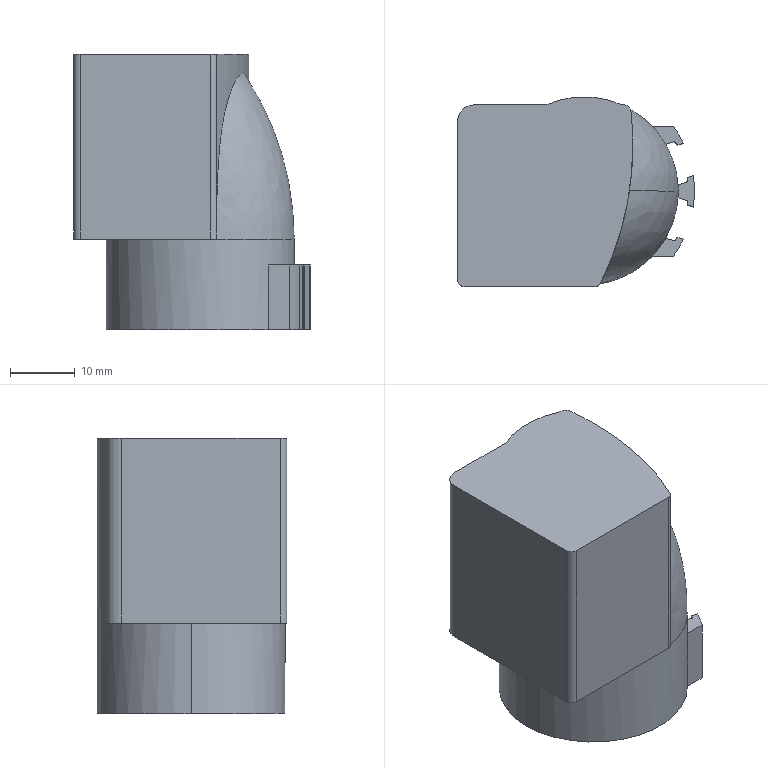Part | STEP file | P393295_cap_HMPL_12 | 1 solid | 62 faces | box 36.5 x 29.25 x 42.5 mm | volume 30561 mm3 | cylinder 34 | plane 24 | spline 2 | cone 2 | commonest cylinder face diameters 0.4 x10 0.8 x4 32 x4 34 x4 2 x3 12.8 x2